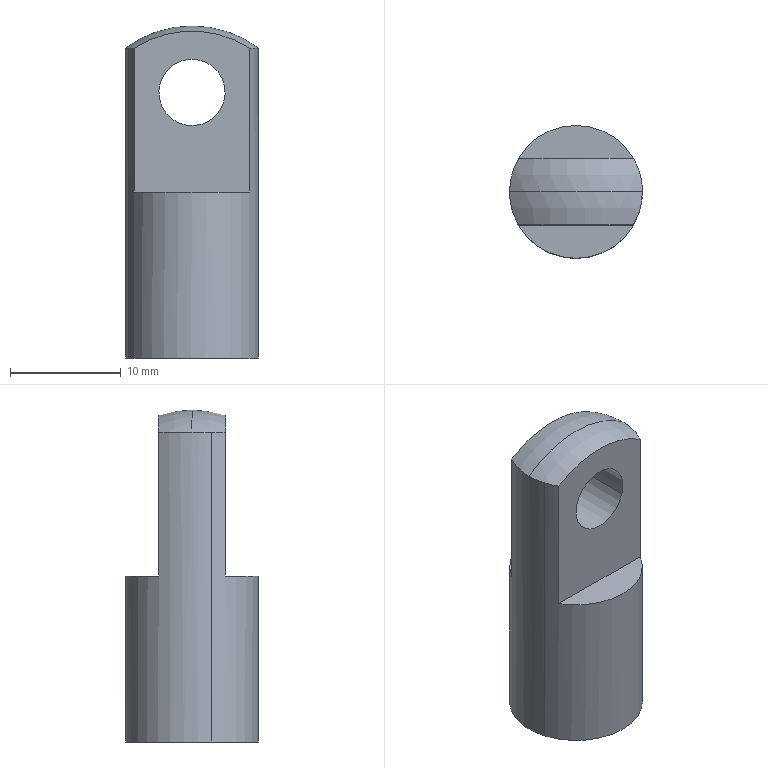Part | SolidWorks | features MBimport 1, MoveFace 1, Scale 1 | 1 solid | 14 faces | box 12 x 12 x 30 mm | volume 1906 mm3 | cylinder 6 | plane 6 | sphere 2 | commonest cylinder face diameters 6 x2 8 x2 12 x2
STEP:
#1=CARTESIAN_POINT('',(-6.,0.,41.073));
#2=VERTEX_POINT('',#1);
#3=CARTESIAN_POINT('',(6.,0.,41.073));
#4=VERTEX_POINT('',#3);
#5=CARTESIAN_POINT('',(0.,0.,33.073));
#6=DIRECTION('',(0.,1.,0.));
#7=DIRECTION('',(0.,0.,-1.));
#8=AXIS2_PLACEMENT_3D('',#5,#6,#7);
#9=CIRCLE('',#8,10.);
#10=EDGE_CURVE('',#2,#4,#9,.T.);
#11=ORIENTED_EDGE('',*,*,#10,.F.);
#12=CARTESIAN_POINT('',(-5.738,-1.754,41.073));
#13=VERTEX_POINT('',#12);
#14=CARTESIAN_POINT('',(0.,0.,41.073));
#15=DIRECTION('',(0.,0.,-1.));
#16=DIRECTION('',(0.9563,0.2924,0.));
#17=AXIS2_PLACEMENT_3D('',#14,#15,#16);
#18=CIRCLE('',#17,6.);
#19=EDGE_CURVE('',#13,#2,#18,.T.);
#20=ORIENTED_EDGE('',*,*,#19,.F.);
#21=CARTESIAN_POINT('',(-5.196,-3.,41.073));
#22=VERTEX_POINT('',#21);
#23=CARTESIAN_POINT('',(0.,0.,41.073));
#24=DIRECTION('',(0.,0.,-1.));
#25=DIRECTION('',(0.9563,0.2924,0.));
#26=AXIS2_PLACEMENT_3D('',#23,#24,#25);
#27=CIRCLE('',#26,6.);
#28=EDGE_CURVE('',#22,#13,#27,.T.);
#29=ORIENTED_EDGE('',*,*,#28,.F.);
#30=CARTESIAN_POINT('',(5.196,-3.,41.073));
#31=VERTEX_POINT('',#30);
#32=CARTESIAN_POINT('',(0.,-3.,33.073));
#33=DIRECTION('',(0.,1.,0.));
#34=DIRECTION('',(0.,0.,-1.));
#35=AXIS2_PLACEMENT_3D('',#32,#33,#34);
#36=CIRCLE('',#35,9.539);
#37=EDGE_CURVE('',#22,#31,#36,.T.);
#38=ORIENTED_EDGE('',*,*,#37,.T.);
#39=CARTESIAN_POINT('',(0.,0.,41.073));
#40=DIRECTION('',(0.,0.,-1.));
#41=DIRECTION('',(0.9563,0.2924,0.));
#42=AXIS2_PLACEMENT_3D('',#39,#40,#41);
#43=CIRCLE('',#42,6.);
#44=EDGE_CURVE('',#4,#31,#43,.T.);
#45=ORIENTED_EDGE('',*,*,#44,.F.);
#46=EDGE_LOOP('',(#11,#20,#29,#38,#45));
#47=FACE_OUTER_BOUND('',#46,.T.);
#48=CARTESIAN_POINT('',(0.,0.,33.073));
#49=DIRECTION('',(0.,-1.,0.));
#50=DIRECTION('',(-1.,0.,0.));
#51=AXIS2_PLACEMENT_3D('',#48,#49,#50);
#52=SPHERICAL_SURFACE('',#51,10.);
#53=ADVANCED_FACE('',(#47),#52,.T.);
#54=CARTESIAN_POINT('',(5.738,1.754,13.073));
#55=VERTEX_POINT('',#54);
#56=CARTESIAN_POINT('',(5.738,1.754,41.073));
#57=VERTEX_POINT('',#56);
#58=CARTESIAN_POINT('',(5.738,1.754,13.073));
#59=DIRECTION('',(0.,0.,1.));
#60=VECTOR('',#59,1000.);
#61=LINE('',#58,#60);
#62=EDGE_CURVE('',#55,#57,#61,.T.);
#63=ORIENTED_EDGE('',*,*,#62,.F.);
#64=CARTESIAN_POINT('',(-5.738,-1.754,13.073));
#65=VERTEX_POINT('',#64);
#66=CARTESIAN_POINT('',(0.,0.,13.073));
#67=DIRECTION('',(0.,0.,1.));
#68=DIRECTION('',(0.9563,0.2924,0.));
#69=AXIS2_PLACEMENT_3D('',#66,#67,#68);
#70=CIRCLE('',#69,6.);
#71=EDGE_CURVE('',#55,#65,#70,.T.);
#72=ORIENTED_EDGE('',*,*,#71,.T.);
#73=CARTESIAN_POINT('',(-5.738,-1.754,13.073));
#74=DIRECTION('',(0.,0.,-1.));
#75=VECTOR('',#74,1000.);
#76=LINE('',#73,#75);
#77=EDGE_CURVE('',#13,#65,#76,.T.);
#78=ORIENTED_EDGE('',*,*,#77,.F.);
#79=ORIENTED_EDGE('',*,*,#19,.T.);
#80=CARTESIAN_POINT('',(-5.196,3.,41.073));
#81=VERTEX_POINT('',#80);
#82=CARTESIAN_POINT('',(0.,0.,41.073));
#83=DIRECTION('',(0.,0.,-1.));
#84=DIRECTION('',(0.9563,0.2924,0.));
#85=AXIS2_PLACEMENT_3D('',#82,#83,#84);
#86=CIRCLE('',#85,6.);
#87=EDGE_CURVE('',#2,#81,#86,.T.);
#88=ORIENTED_EDGE('',*,*,#87,.T.);
#89=CARTESIAN_POINT('',(-5.196,3.,28.073));
#90=VERTEX_POINT('',#89);
#91=CARTESIAN_POINT('',(-5.196,3.,34.573));
#92=DIRECTION('',(0.,0.,-1.));
#93=VECTOR('',#92,1000.);
#94=LINE('',#91,#93);
#95=EDGE_CURVE('',#81,#90,#94,.T.);
#96=ORIENTED_EDGE('',*,*,#95,.T.);
#97=CARTESIAN_POINT('',(5.196,3.,28.073));
#98=VERTEX_POINT('',#97);
#99=CARTESIAN_POINT('',(0.,0.,28.073));
#100=DIRECTION('',(0.,0.,-1.));
#101=DIRECTION('',(0.9563,0.2924,0.));
#102=AXIS2_PLACEMENT_3D('',#99,#100,#101);
#103=CIRCLE('',#102,6.);
#104=EDGE_CURVE('',#90,#98,#103,.T.);
#105=ORIENTED_EDGE('',*,*,#104,.T.);
#106=CARTESIAN_POINT('',(5.196,3.,41.073));
#107=VERTEX_POINT('',#106);
#108=CARTESIAN_POINT('',(5.196,3.,34.573));
#109=DIRECTION('',(0.,0.,1.));
#110=VECTOR('',#109,1000.);
#111=LINE('',#108,#110);
#112=EDGE_CURVE('',#98,#107,#111,.T.);
#113=ORIENTED_EDGE('',*,*,#112,.T.);
#114=CARTESIAN_POINT('',(0.,0.,41.073));
#115=DIRECTION('',(0.,0.,-1.));
#116=DIRECTION('',(0.9563,0.2924,0.));
#117=AXIS2_PLACEMENT_3D('',#114,#115,#116);
#118=CIRCLE('',#117,6.);
#119=EDGE_CURVE('',#107,#57,#118,.T.);
#120=ORIENTED_EDGE('',*,*,#119,.T.);
#121=EDGE_LOOP('',(#63,#72,#78,#79,#88,#96,#105,#113,#120));
#122=FACE_OUTER_BOUND('',#121,.T.);
#123=CARTESIAN_POINT('',(0.,0.,13.073));
#124=DIRECTION('',(0.,0.,1.));
#125=DIRECTION('',(-0.9563,-0.2924,0.));
#126=AXIS2_PLACEMENT_3D('',#123,#124,#125);
#127=CYLINDRICAL_SURFACE('',#126,6.);
#128=ADVANCED_FACE('',(#122),#127,.T.);
#129=CARTESIAN_POINT('',(-2.869,-3.,37.95));
#130=VERTEX_POINT('',#129);
#131=CARTESIAN_POINT('',(-2.869,3.,37.95));
#132=VERTEX_POINT('',#131);
#133=CARTESIAN_POINT('',(-2.869,3.,37.95));
#134=DIRECTION('',(0.,1.,0.));
#135=VECTOR('',#134,1000.);
#136=LINE('',#133,#135);
#137=EDGE_CURVE('',#130,#132,#136,.T.);
#138=ORIENTED_EDGE('',*,*,#137,.F.);
#139=CARTESIAN_POINT('',(2.869,-3.,36.195));
#140=VERTEX_POINT('',#139);
#141=CARTESIAN_POINT('',(0.,-3.,37.073));
#142=DIRECTION('',(0.,1.,0.));
#143=DIRECTION('',(-0.9563,0.,0.2924));
#144=AXIS2_PLACEMENT_3D('',#141,#142,#143);
#145=CIRCLE('',#144,3.);
#146=EDGE_CURVE('',#140,#130,#145,.T.);
#147=ORIENTED_EDGE('',*,*,#146,.F.);
#148=CARTESIAN_POINT('',(2.869,3.,36.195));
#149=VERTEX_POINT('',#148);
#150=CARTESIAN_POINT('',(2.869,3.,36.195));
#151=DIRECTION('',(0.,-1.,0.));
#152=VECTOR('',#151,1000.);
#153=LINE('',#150,#152);
#154=EDGE_CURVE('',#149,#140,#153,.T.);
#155=ORIENTED_EDGE('',*,*,#154,.F.);
#156=CARTESIAN_POINT('',(0.,3.,37.073));
#157=DIRECTION('',(0.,-1.,0.));
#158=DIRECTION('',(-0.9563,0.,0.2924));
#159=AXIS2_PLACEMENT_3D('',#156,#157,#158);
#160=CIRCLE('',#159,3.);
#161=EDGE_CURVE('',#132,#149,#160,.T.);
#162=ORIENTED_EDGE('',*,*,#161,.F.);
#163=EDGE_LOOP('',(#138,#147,#155,#162));
#164=FACE_OUTER_BOUND('',#163,.T.);
#165=CARTESIAN_POINT('',(0.,3.,37.073));
#166=DIRECTION('',(0.,-1.,0.));
#167=DIRECTION('',(0.9563,0.,-0.2924));
#168=AXIS2_PLACEMENT_3D('',#165,#166,#167);
#169=CYLINDRICAL_SURFACE('',#168,3.);
#170=ADVANCED_FACE('',(#164),#169,.F.);
#171=CARTESIAN_POINT('',(-3.825,1.169,25.073));
#172=VERTEX_POINT('',#171);
#173=CARTESIAN_POINT('',(-3.825,1.169,13.073));
#174=VERTEX_POINT('',#173);
#175=CARTESIAN_POINT('',(-3.825,1.169,13.073));
#176=DIRECTION('',(0.,0.,-1.));
#177=VECTOR('',#176,1000.);
#178=LINE('',#175,#177);
#179=EDGE_CURVE('',#172,#174,#178,.T.);
#180=ORIENTED_EDGE('',*,*,#179,.F.);
#181=CARTESIAN_POINT('',(3.825,-1.169,25.073));
#182=VERTEX_POINT('',#181);
#183=CARTESIAN_POINT('',(0.,0.,25.073));
#184=DIRECTION('',(0.,0.,-1.));
#185=DIRECTION('',(-1.,0.,0.));
#186=AXIS2_PLACEMENT_3D('',#183,#184,#185);
#187=CIRCLE('',#186,4.);
#188=EDGE_CURVE('',#182,#172,#187,.T.);
#189=ORIENTED_EDGE('',*,*,#188,.F.);
#190=CARTESIAN_POINT('',(3.825,-1.169,13.073));
#191=VERTEX_POINT('',#190);
#192=CARTESIAN_POINT('',(3.825,-1.169,13.073));
#193=DIRECTION('',(0.,0.,1.));
#194=VECTOR('',#193,1000.);
#195=LINE('',#192,#194);
#196=EDGE_CURVE('',#191,#182,#195,.T.);
#197=ORIENTED_EDGE('',*,*,#196,.F.);
#198=CARTESIAN_POINT('',(0.,0.,13.073));
#199=DIRECTION('',(0.,0.,1.));
#200=DIRECTION('',(1.,0.,0.));
#201=AXIS2_PLACEMENT_3D('',#198,#199,#200);
#202=CIRCLE('',#201,4.);
#203=EDGE_CURVE('',#174,#191,#202,.T.);
#204=ORIENTED_EDGE('',*,*,#203,.F.);
#205=EDGE_LOOP('',(#180,#189,#197,#204));
#206=FACE_OUTER_BOUND('',#205,.T.);
#207=CARTESIAN_POINT('',(0.,0.,13.073));
#208=DIRECTION('',(0.,0.,1.));
#209=DIRECTION('',(0.9563,-0.2924,0.));
#210=AXIS2_PLACEMENT_3D('',#207,#208,#209);
#211=CYLINDRICAL_SURFACE('',#210,4.);
#212=ADVANCED_FACE('',(#206),#211,.F.);
#213=CARTESIAN_POINT('',(0.,0.,25.073));
#214=DIRECTION('',(0.,0.,-1.));
#215=DIRECTION('',(-1.,0.,0.));
#216=AXIS2_PLACEMENT_3D('',#213,#214,#215);
#217=CIRCLE('',#216,4.);
#218=EDGE_CURVE('',#172,#182,#217,.T.);
#219=ORIENTED_EDGE('',*,*,#218,.T.);
#220=ORIENTED_EDGE('',*,*,#188,.T.);
#221=EDGE_LOOP('',(#219,#220));
#222=FACE_OUTER_BOUND('',#221,.T.);
#223=CARTESIAN_POINT('',(0.,0.,25.073));
#224=DIRECTION('',(0.,0.,-1.));
#225=DIRECTION('',(0.,-1.,0.));
#226=AXIS2_PLACEMENT_3D('',#223,#224,#225);
#227=PLANE('',#226);
#228=ADVANCED_FACE('',(#222),#227,.T.);
#229=ORIENTED_EDGE('',*,*,#179,.T.);
#230=CARTESIAN_POINT('',(0.,0.,13.073));
#231=DIRECTION('',(0.,0.,1.));
#232=DIRECTION('',(1.,0.,0.));
#233=AXIS2_PLACEMENT_3D('',#230,#231,#232);
#234=CIRCLE('',#233,4.);
#235=EDGE_CURVE('',#191,#174,#234,.T.);
#236=ORIENTED_EDGE('',*,*,#235,.F.);
#237=ORIENTED_EDGE('',*,*,#196,.T.);
#238=ORIENTED_EDGE('',*,*,#218,.F.);
#239=EDGE_LOOP('',(#229,#236,#237,#238));
#240=FACE_OUTER_BOUND('',#239,.T.);
#241=CARTESIAN_POINT('',(0.,0.,13.073));
#242=DIRECTION('',(0.,0.,1.));
#243=DIRECTION('',(0.9563,-0.2924,0.));
#244=AXIS2_PLACEMENT_3D('',#241,#242,#243);
#245=CYLINDRICAL_SURFACE('',#244,4.);
#246=ADVANCED_FACE('',(#240),#245,.F.);
#247=ORIENTED_EDGE('',*,*,#137,.T.);
#248=CARTESIAN_POINT('',(0.,3.,37.073));
#249=DIRECTION('',(0.,-1.,0.));
#250=DIRECTION('',(-0.9563,0.,0.2924));
#251=AXIS2_PLACEMENT_3D('',#248,#249,#250);
#252=CIRCLE('',#251,3.);
#253=EDGE_CURVE('',#149,#132,#252,.T.);
#254=ORIENTED_EDGE('',*,*,#253,.F.);
#255=ORIENTED_EDGE('',*,*,#154,.T.);
#256=CARTESIAN_POINT('',(0.,-3.,37.073));
#257=DIRECTION('',(0.,1.,0.));
#258=DIRECTION('',(-0.9563,0.,0.2924));
#259=AXIS2_PLACEMENT_3D('',#256,#257,#258);
#260=CIRCLE('',#259,3.);
#261=EDGE_CURVE('',#130,#140,#260,.T.);
#262=ORIENTED_EDGE('',*,*,#261,.F.);
#263=EDGE_LOOP('',(#247,#254,#255,#262));
#264=FACE_OUTER_BOUND('',#263,.T.);
#265=CARTESIAN_POINT('',(0.,3.,37.073));
#266=DIRECTION('',(0.,-1.,0.));
#267=DIRECTION('',(0.9563,0.,-0.2924));
#268=AXIS2_PLACEMENT_3D('',#265,#266,#267);
#269=CYLINDRICAL_SURFACE('',#268,3.);
#270=ADVANCED_FACE('',(#264),#269,.F.);
#271=CARTESIAN_POINT('',(5.196,-3.,28.073));
#272=VERTEX_POINT('',#271);
#273=CARTESIAN_POINT('',(-5.196,-3.,28.073));
#274=VERTEX_POINT('',#273);
#275=CARTESIAN_POINT('',(0.,0.,28.073));
#276=DIRECTION('',(0.,0.,-1.));
#277=DIRECTION('',(0.9563,0.2924,0.));
#278=AXIS2_PLACEMENT_3D('',#275,#276,#277);
#279=CIRCLE('',#278,6.);
#280=EDGE_CURVE('',#272,#274,#279,.T.);
#281=ORIENTED_EDGE('',*,*,#280,.F.);
#282=CARTESIAN_POINT('',(0.,-3.,28.073));
#283=DIRECTION('',(1.,0.,0.));
#284=VECTOR('',#283,1000.);
#285=LINE('',#282,#284);
#286=EDGE_CURVE('',#274,#272,#285,.T.);
#287=ORIENTED_EDGE('',*,*,#286,.F.);
#288=EDGE_LOOP('',(#281,#287));
#289=FACE_OUTER_BOUND('',#288,.T.);
#290=CARTESIAN_POINT('',(0.,-6.,28.073));
#291=DIRECTION('',(0.,0.,-1.));
#292=DIRECTION('',(0.,-1.,0.));
#293=AXIS2_PLACEMENT_3D('',#290,#291,#292);
#294=PLANE('',#293);
#295=ADVANCED_FACE('',(#289),#294,.F.);
#296=ORIENTED_EDGE('',*,*,#146,.T.);
#297=ORIENTED_EDGE('',*,*,#261,.T.);
#298=EDGE_LOOP('',(#296,#297));
#299=FACE_BOUND('',#298,.T.);
#300=CARTESIAN_POINT('',(5.196,-3.,34.573));
#301=DIRECTION('',(0.,0.,-1.));
#302=VECTOR('',#301,1000.);
#303=LINE('',#300,#302);
#304=EDGE_CURVE('',#31,#272,#303,.T.);
#305=ORIENTED_EDGE('',*,*,#304,.F.);
#306=ORIENTED_EDGE('',*,*,#37,.F.);
#307=CARTESIAN_POINT('',(-5.196,-3.,34.573));
#308=DIRECTION('',(0.,0.,1.));
#309=VECTOR('',#308,1000.);
#310=LINE('',#307,#309);
#311=EDGE_CURVE('',#274,#22,#310,.T.);
#312=ORIENTED_EDGE('',*,*,#311,.F.);
#313=ORIENTED_EDGE('',*,*,#286,.T.);
#314=EDGE_LOOP('',(#305,#306,#312,#313));
#315=FACE_OUTER_BOUND('',#314,.T.);
#316=CARTESIAN_POINT('',(0.,-3.,37.073));
#317=DIRECTION('',(0.,1.,0.));
#318=DIRECTION('',(1.,0.,0.));
#319=AXIS2_PLACEMENT_3D('',#316,#317,#318);
#320=PLANE('',#319);
#321=ADVANCED_FACE('',(#299,#315),#320,.F.);
#322=ORIENTED_EDGE('',*,*,#104,.F.);
#323=CARTESIAN_POINT('',(0.,3.,28.073));
#324=DIRECTION('',(-1.,0.,0.));
#325=VECTOR('',#324,1000.);
#326=LINE('',#323,#325);
#327=EDGE_CURVE('',#98,#90,#326,.T.);
#328=ORIENTED_EDGE('',*,*,#327,.F.);
#329=EDGE_LOOP('',(#322,#328));
#330=FACE_OUTER_BOUND('',#329,.T.);
#331=CARTESIAN_POINT('',(0.,6.,28.073));
#332=DIRECTION('',(0.,0.,-1.));
#333=DIRECTION('',(0.,-1.,0.));
#334=AXIS2_PLACEMENT_3D('',#331,#332,#333);
#335=PLANE('',#334);
#336=ADVANCED_FACE('',(#330),#335,.F.);
#337=ORIENTED_EDGE('',*,*,#253,.T.);
#338=ORIENTED_EDGE('',*,*,#161,.T.);
#339=EDGE_LOOP('',(#337,#338));
#340=FACE_BOUND('',#339,.T.);
#341=ORIENTED_EDGE('',*,*,#95,.F.);
#342=CARTESIAN_POINT('',(0.,3.,33.073));
#343=DIRECTION('',(0.,-1.,0.));
#344=DIRECTION('',(0.,0.,1.));
#345=AXIS2_PLACEMENT_3D('',#342,#343,#344);
#346=CIRCLE('',#345,9.539);
#347=EDGE_CURVE('',#107,#81,#346,.T.);
#348=ORIENTED_EDGE('',*,*,#347,.F.);
#349=ORIENTED_EDGE('',*,*,#112,.F.);
#350=ORIENTED_EDGE('',*,*,#327,.T.);
#351=EDGE_LOOP('',(#341,#348,#349,#350));
#352=FACE_OUTER_BOUND('',#351,.T.);
#353=CARTESIAN_POINT('',(0.,3.,37.073));
#354=DIRECTION('',(0.,-1.,0.));
#355=DIRECTION('',(0.,0.,-1.));
#356=AXIS2_PLACEMENT_3D('',#353,#354,#355);
#357=PLANE('',#356);
#358=ADVANCED_FACE('',(#340,#352),#357,.F.);
#359=ORIENTED_EDGE('',*,*,#62,.T.);
#360=CARTESIAN_POINT('',(0.,0.,41.073));
#361=DIRECTION('',(0.,0.,-1.));
#362=DIRECTION('',(0.9563,0.2924,0.));
#363=AXIS2_PLACEMENT_3D('',#360,#361,#362);
#364=CIRCLE('',#363,6.);
#365=EDGE_CURVE('',#57,#4,#364,.T.);
#366=ORIENTED_EDGE('',*,*,#365,.T.);
#367=ORIENTED_EDGE('',*,*,#44,.T.);
#368=ORIENTED_EDGE('',*,*,#304,.T.);
#369=ORIENTED_EDGE('',*,*,#280,.T.);
#370=ORIENTED_EDGE('',*,*,#311,.T.);
#371=ORIENTED_EDGE('',*,*,#28,.T.);
#372=ORIENTED_EDGE('',*,*,#77,.T.);
#373=CARTESIAN_POINT('',(0.,0.,13.073));
#374=DIRECTION('',(0.,0.,1.));
#375=DIRECTION('',(0.9563,0.2924,0.));
#376=AXIS2_PLACEMENT_3D('',#373,#374,#375);
#377=CIRCLE('',#376,6.);
#378=EDGE_CURVE('',#65,#55,#377,.T.);
#379=ORIENTED_EDGE('',*,*,#378,.T.);
#380=EDGE_LOOP('',(#359,#366,#367,#368,#369,#370,#371,#372,#379));
#381=FACE_OUTER_BOUND('',#380,.T.);
#382=CARTESIAN_POINT('',(0.,0.,13.073));
#383=DIRECTION('',(0.,0.,1.));
#384=DIRECTION('',(-0.9563,-0.2924,0.));
#385=AXIS2_PLACEMENT_3D('',#382,#383,#384);
#386=CYLINDRICAL_SURFACE('',#385,6.);
#387=ADVANCED_FACE('',(#381),#386,.T.);
#388=ORIENTED_EDGE('',*,*,#10,.T.);
#389=ORIENTED_EDGE('',*,*,#365,.F.);
#390=ORIENTED_EDGE('',*,*,#119,.F.);
#391=ORIENTED_EDGE('',*,*,#347,.T.);
#392=ORIENTED_EDGE('',*,*,#87,.F.);
#393=EDGE_LOOP('',(#388,#389,#390,#391,#392));
#394=FACE_OUTER_BOUND('',#393,.T.);
#395=CARTESIAN_POINT('',(0.,0.,33.073));
#396=DIRECTION('',(0.,-1.,0.));
#397=DIRECTION('',(-1.,0.,0.));
#398=AXIS2_PLACEMENT_3D('',#395,#396,#397);
#399=SPHERICAL_SURFACE('',#398,10.);
#400=ADVANCED_FACE('',(#394),#399,.T.);
#401=ORIENTED_EDGE('',*,*,#203,.T.);
#402=ORIENTED_EDGE('',*,*,#235,.T.);
#403=EDGE_LOOP('',(#401,#402));
#404=FACE_BOUND('',#403,.T.);
#405=ORIENTED_EDGE('',*,*,#71,.F.);
#406=ORIENTED_EDGE('',*,*,#378,.F.);
#407=EDGE_LOOP('',(#405,#406));
#408=FACE_OUTER_BOUND('',#407,.T.);
#409=CARTESIAN_POINT('',(0.,0.,13.073));
#410=DIRECTION('',(0.,0.,1.));
#411=DIRECTION('',(1.,0.,0.));
#412=AXIS2_PLACEMENT_3D('',#409,#410,#411);
#413=PLANE('',#412);
#414=ADVANCED_FACE('',(#404,#408),#413,.F.);
#415=CLOSED_SHELL('',(#53,#128,#170,#212,#228,#246,#270,#295,#321,#336,#358,#387,#400,#414));
#416=MANIFOLD_SOLID_BREP('',#415);
#417=CARTESIAN_POINT('',(0.,0.,0.));
#418=DIRECTION('',(0.,0.,1.));
#419=DIRECTION('',(1.,0.,0.));
#420=AXIS2_PLACEMENT_3D('',#417,#418,#419);
#421=(LENGTH_UNIT()NAMED_UNIT(*)SI_UNIT(.MILLI.,.METRE.));
#422=UNCERTAINTY_MEASURE_WITH_UNIT(LENGTH_MEASURE(0.00001),#421,'','');
#423=(NAMED_UNIT(*)PLANE_ANGLE_UNIT()SI_UNIT($,.RADIAN.));
#424=(NAMED_UNIT(*)SI_UNIT($,.STERADIAN.)SOLID_ANGLE_UNIT());
#425=(GEOMETRIC_REPRESENTATION_CONTEXT(3)GLOBAL_UNCERTAINTY_ASSIGNED_CONTEXT((#422))GLOBAL_UNIT_ASSIGNED_CONTEXT((#421,#423,#424))REPRESENTATION_CONTEXT('',''));
#426=ADVANCED_BREP_SHAPE_REPRESENTATION('',(#416,#420),#425);